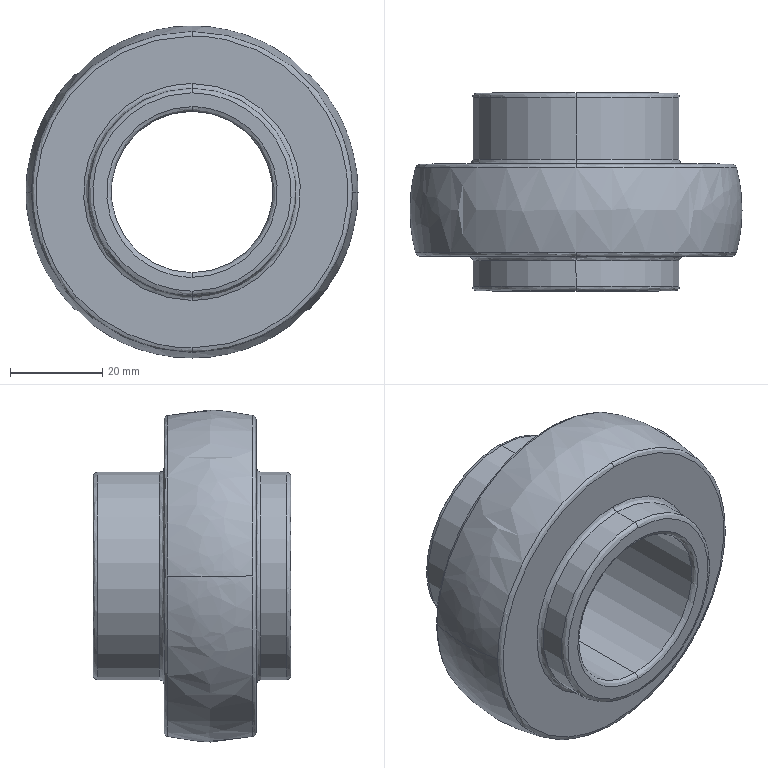Part | SolidWorks | features BaseBody 1 | 1 solid | 28 faces | volume 74359 mm3 | spline 18 | cylinder 6 | plane 4 | commonest cylinder face diameters 45 x4 35 x2